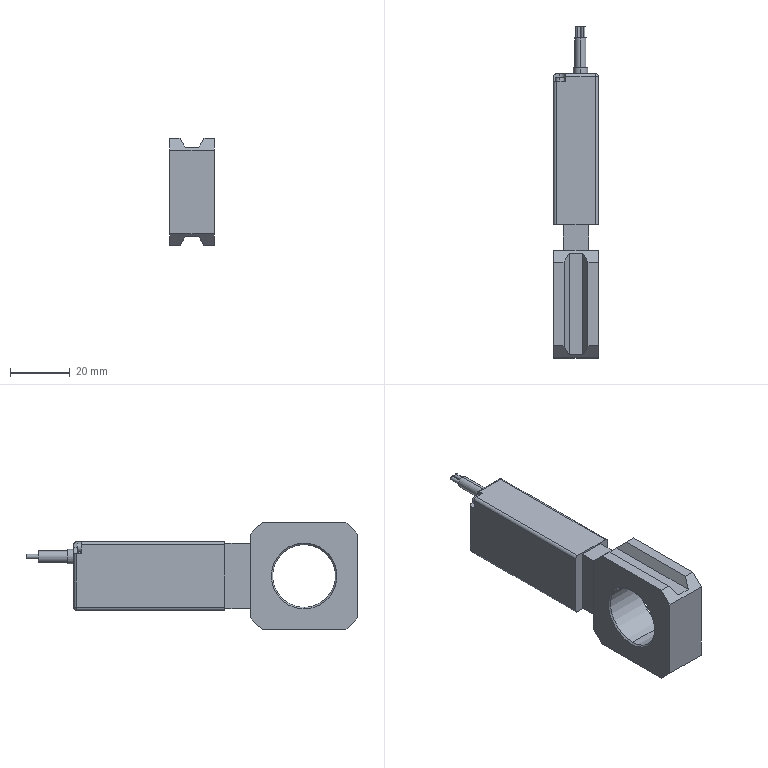Part | STEP file | AC40-04-KSTV-38JNR_AC3009A Switch | 1 solid | 70 faces | box 15 x 111 x 36 mm | volume 31675 mm3 | plane 40 | cylinder 24 | cone 4 | sphere 2 | commonest cylinder face diameters 2 x8 1.5 x4 3 x4 3.8 x2 4 x2 4.8 x2